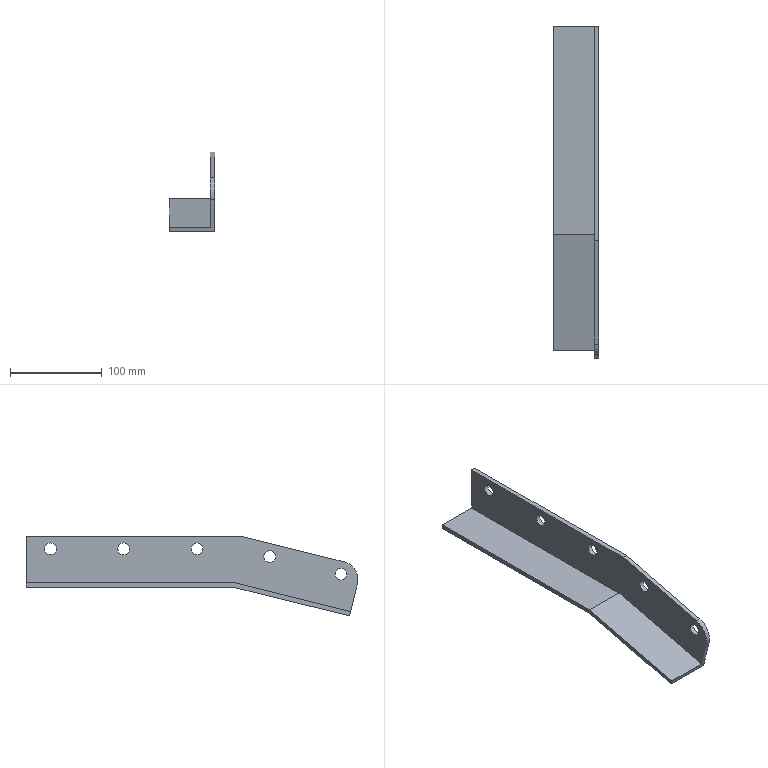Part | NX | features solid 2 | 1 solid | 17 faces | box 50 x 362.429 x 87.264 mm | volume 178588 mm3 | plane 11 | cylinder 6 | commonest cylinder face diameters 13 x5 40 x1
STEP:
#1=CARTESIAN_POINT('',(-584.258,-720.,106.));
#2=VERTEX_POINT('',#1);
#3=CARTESIAN_POINT('',(-584.258,-720.,55.));
#4=VERTEX_POINT('',#3);
#5=CARTESIAN_POINT('',(-584.258,-720.,85.));
#6=DIRECTION('',(0.,0.,-1.));
#7=VECTOR('',#6,1000.);
#8=LINE('',#5,#7);
#9=EDGE_CURVE('',#2,#4,#8,.T.);
#10=ORIENTED_EDGE('',*,*,#9,.F.);
#11=CARTESIAN_POINT('',(-579.258,-720.,106.));
#12=VERTEX_POINT('',#11);
#13=CARTESIAN_POINT('',(-584.258,-720.,106.));
#14=DIRECTION('',(-1.,0.,0.));
#15=VECTOR('',#14,1000.);
#16=LINE('',#13,#15);
#17=EDGE_CURVE('',#12,#2,#16,.T.);
#18=ORIENTED_EDGE('',*,*,#17,.F.);
#19=CARTESIAN_POINT('',(-579.258,-720.,50.));
#20=VERTEX_POINT('',#19);
#21=CARTESIAN_POINT('',(-579.258,-720.,85.));
#22=DIRECTION('',(0.,0.,1.));
#23=VECTOR('',#22,1000.);
#24=LINE('',#21,#23);
#25=EDGE_CURVE('',#20,#12,#24,.T.);
#26=ORIENTED_EDGE('',*,*,#25,.F.);
#27=CARTESIAN_POINT('',(-629.258,-720.,50.));
#28=VERTEX_POINT('',#27);
#29=CARTESIAN_POINT('',(-579.258,-720.,50.));
#30=DIRECTION('',(1.,0.,0.));
#31=VECTOR('',#30,1000.);
#32=LINE('',#29,#31);
#33=EDGE_CURVE('',#28,#20,#32,.T.);
#34=ORIENTED_EDGE('',*,*,#33,.F.);
#35=CARTESIAN_POINT('',(-629.258,-720.,55.));
#36=VERTEX_POINT('',#35);
#37=CARTESIAN_POINT('',(-629.258,-720.,85.));
#38=DIRECTION('',(0.,0.,-1.));
#39=VECTOR('',#38,1000.);
#40=LINE('',#37,#39);
#41=EDGE_CURVE('',#36,#28,#40,.T.);
#42=ORIENTED_EDGE('',*,*,#41,.F.);
#43=CARTESIAN_POINT('',(-624.258,-720.,55.));
#44=DIRECTION('',(-1.,0.,0.));
#45=VECTOR('',#44,1000.);
#46=LINE('',#43,#45);
#47=EDGE_CURVE('',#4,#36,#46,.T.);
#48=ORIENTED_EDGE('',*,*,#47,.F.);
#49=EDGE_LOOP('',(#10,#18,#26,#34,#42,#48));
#50=FACE_BOUND('',#49,.T.);
#51=CARTESIAN_POINT('',(-1045.,-720.,130.));
#52=DIRECTION('',(0.,1.,0.));
#53=DIRECTION('',(0.,0.,1.));
#54=AXIS2_PLACEMENT_3D('',#51,#52,#53);
#55=PLANE('',#54);
#56=ADVANCED_FACE('',(#50),#55,.T.);
#57=CARTESIAN_POINT('',(-584.258,-1063.872,70.813));
#58=VERTEX_POINT('',#57);
#59=CARTESIAN_POINT('',(-584.258,-1063.872,64.313));
#60=DIRECTION('',(1.,0.,0.));
#61=DIRECTION('',(0.,0.,1.));
#62=AXIS2_PLACEMENT_3D('',#59,#60,#61);
#63=CIRCLE('',#62,6.5);
#64=EDGE_CURVE('',#58,#58,#63,.T.);
#65=ORIENTED_EDGE('',*,*,#64,.T.);
#66=EDGE_LOOP('',(#65));
#67=FACE_BOUND('',#66,.T.);
#68=CARTESIAN_POINT('',(-584.258,-986.22,90.053));
#69=VERTEX_POINT('',#68);
#70=CARTESIAN_POINT('',(-584.258,-986.22,83.553));
#71=DIRECTION('',(1.,0.,0.));
#72=DIRECTION('',(0.,0.,1.));
#73=AXIS2_PLACEMENT_3D('',#70,#71,#72);
#74=CIRCLE('',#73,6.5);
#75=EDGE_CURVE('',#69,#69,#74,.T.);
#76=ORIENTED_EDGE('',*,*,#75,.T.);
#77=EDGE_LOOP('',(#76));
#78=FACE_BOUND('',#77,.T.);
#79=CARTESIAN_POINT('',(-584.258,-906.667,98.5));
#80=VERTEX_POINT('',#79);
#81=CARTESIAN_POINT('',(-584.258,-906.667,92.));
#82=DIRECTION('',(1.,0.,0.));
#83=DIRECTION('',(0.,0.,1.));
#84=AXIS2_PLACEMENT_3D('',#81,#82,#83);
#85=CIRCLE('',#84,6.5);
#86=EDGE_CURVE('',#80,#80,#85,.T.);
#87=ORIENTED_EDGE('',*,*,#86,.T.);
#88=EDGE_LOOP('',(#87));
#89=FACE_BOUND('',#88,.T.);
#90=CARTESIAN_POINT('',(-584.258,-826.667,98.5));
#91=VERTEX_POINT('',#90);
#92=CARTESIAN_POINT('',(-584.258,-826.667,92.));
#93=DIRECTION('',(1.,0.,0.));
#94=DIRECTION('',(0.,0.,1.));
#95=AXIS2_PLACEMENT_3D('',#92,#93,#94);
#96=CIRCLE('',#95,6.5);
#97=EDGE_CURVE('',#91,#91,#96,.T.);
#98=ORIENTED_EDGE('',*,*,#97,.T.);
#99=EDGE_LOOP('',(#98));
#100=FACE_BOUND('',#99,.T.);
#101=CARTESIAN_POINT('',(-584.258,-746.667,98.5));
#102=VERTEX_POINT('',#101);
#103=CARTESIAN_POINT('',(-584.258,-746.667,92.));
#104=DIRECTION('',(1.,0.,0.));
#105=DIRECTION('',(0.,0.,1.));
#106=AXIS2_PLACEMENT_3D('',#103,#104,#105);
#107=CIRCLE('',#106,6.5);
#108=EDGE_CURVE('',#102,#102,#107,.T.);
#109=ORIENTED_EDGE('',*,*,#108,.T.);
#110=EDGE_LOOP('',(#109));
#111=FACE_BOUND('',#110,.T.);
#112=CARTESIAN_POINT('',(-584.258,-953.834,106.));
#113=VERTEX_POINT('',#112);
#114=CARTESIAN_POINT('',(-584.258,-904.636,106.));
#115=DIRECTION('',(0.,-1.,0.));
#116=VECTOR('',#115,1000.);
#117=LINE('',#114,#116);
#118=EDGE_CURVE('',#2,#113,#117,.T.);
#119=ORIENTED_EDGE('',*,*,#118,.F.);
#120=ORIENTED_EDGE('',*,*,#9,.T.);
#121=CARTESIAN_POINT('',(-584.258,-947.61,55.));
#122=VERTEX_POINT('',#121);
#123=CARTESIAN_POINT('',(-584.258,-902.805,55.));
#124=DIRECTION('',(0.,-1.,0.));
#125=VECTOR('',#124,1000.);
#126=LINE('',#123,#125);
#127=EDGE_CURVE('',#4,#122,#126,.T.);
#128=ORIENTED_EDGE('',*,*,#127,.T.);
#129=CARTESIAN_POINT('',(-584.258,-1074.387,23.589));
#130=VERTEX_POINT('',#129);
#131=CARTESIAN_POINT('',(-584.258,-997.906,42.538));
#132=DIRECTION('',(0.,-0.9707,-0.2405));
#133=VECTOR('',#132,1000.);
#134=LINE('',#131,#133);
#135=EDGE_CURVE('',#122,#130,#134,.T.);
#136=ORIENTED_EDGE('',*,*,#135,.T.);
#137=CARTESIAN_POINT('',(-584.258,-1081.842,53.679));
#138=VERTEX_POINT('',#137);
#139=CARTESIAN_POINT('',(-584.258,-1073.185,18.736));
#140=DIRECTION('',(0.,0.2405,-0.9707));
#141=VECTOR('',#140,1000.);
#142=LINE('',#139,#141);
#143=EDGE_CURVE('',#138,#130,#142,.T.);
#144=ORIENTED_EDGE('',*,*,#143,.F.);
#145=CARTESIAN_POINT('',(-584.258,-1067.239,77.902));
#146=VERTEX_POINT('',#145);
#147=CARTESIAN_POINT('',(-584.258,-1062.429,58.489));
#148=DIRECTION('',(-1.,0.,0.));
#149=DIRECTION('',(0.,0.,-1.));
#150=AXIS2_PLACEMENT_3D('',#147,#148,#149);
#151=CIRCLE('',#150,20.);
#152=EDGE_CURVE('',#138,#146,#151,.T.);
#153=ORIENTED_EDGE('',*,*,#152,.T.);
#154=CARTESIAN_POINT('',(-584.258,-1008.395,92.482));
#155=DIRECTION('',(0.,-0.9707,-0.2405));
#156=VECTOR('',#155,1000.);
#157=LINE('',#154,#156);
#158=EDGE_CURVE('',#113,#146,#157,.T.);
#159=ORIENTED_EDGE('',*,*,#158,.F.);
#160=EDGE_LOOP('',(#119,#120,#128,#136,#144,#153,#159));
#161=FACE_BOUND('',#160,.T.);
#162=CARTESIAN_POINT('',(-584.258,-904.636,85.));
#163=DIRECTION('',(-1.,0.,0.));
#164=DIRECTION('',(0.,0.,-1.));
#165=AXIS2_PLACEMENT_3D('',#162,#163,#164);
#166=PLANE('',#165);
#167=ADVANCED_FACE('',(#67,#78,#89,#100,#111,#161),#166,.T.);
#168=CARTESIAN_POINT('',(-579.258,-1063.872,70.813));
#169=VERTEX_POINT('',#168);
#170=CARTESIAN_POINT('',(-579.258,-1063.872,64.313));
#171=DIRECTION('',(1.,0.,0.));
#172=DIRECTION('',(0.,0.,1.));
#173=AXIS2_PLACEMENT_3D('',#170,#171,#172);
#174=CIRCLE('',#173,6.5);
#175=EDGE_CURVE('',#169,#169,#174,.T.);
#176=ORIENTED_EDGE('',*,*,#175,.F.);
#177=EDGE_LOOP('',(#176));
#178=FACE_BOUND('',#177,.T.);
#179=CARTESIAN_POINT('',(-579.258,-986.22,90.053));
#180=VERTEX_POINT('',#179);
#181=CARTESIAN_POINT('',(-579.258,-986.22,83.553));
#182=DIRECTION('',(1.,0.,0.));
#183=DIRECTION('',(0.,0.,1.));
#184=AXIS2_PLACEMENT_3D('',#181,#182,#183);
#185=CIRCLE('',#184,6.5);
#186=EDGE_CURVE('',#180,#180,#185,.T.);
#187=ORIENTED_EDGE('',*,*,#186,.F.);
#188=EDGE_LOOP('',(#187));
#189=FACE_BOUND('',#188,.T.);
#190=CARTESIAN_POINT('',(-579.258,-906.667,98.5));
#191=VERTEX_POINT('',#190);
#192=CARTESIAN_POINT('',(-579.258,-906.667,92.));
#193=DIRECTION('',(1.,0.,0.));
#194=DIRECTION('',(0.,0.,1.));
#195=AXIS2_PLACEMENT_3D('',#192,#193,#194);
#196=CIRCLE('',#195,6.5);
#197=EDGE_CURVE('',#191,#191,#196,.T.);
#198=ORIENTED_EDGE('',*,*,#197,.F.);
#199=EDGE_LOOP('',(#198));
#200=FACE_BOUND('',#199,.T.);
#201=CARTESIAN_POINT('',(-579.258,-826.667,98.5));
#202=VERTEX_POINT('',#201);
#203=CARTESIAN_POINT('',(-579.258,-826.667,92.));
#204=DIRECTION('',(1.,0.,0.));
#205=DIRECTION('',(0.,0.,1.));
#206=AXIS2_PLACEMENT_3D('',#203,#204,#205);
#207=CIRCLE('',#206,6.5);
#208=EDGE_CURVE('',#202,#202,#207,.T.);
#209=ORIENTED_EDGE('',*,*,#208,.F.);
#210=EDGE_LOOP('',(#209));
#211=FACE_BOUND('',#210,.T.);
#212=CARTESIAN_POINT('',(-579.258,-746.667,98.5));
#213=VERTEX_POINT('',#212);
#214=CARTESIAN_POINT('',(-579.258,-746.667,92.));
#215=DIRECTION('',(1.,0.,0.));
#216=DIRECTION('',(0.,0.,1.));
#217=AXIS2_PLACEMENT_3D('',#214,#215,#216);
#218=CIRCLE('',#217,6.5);
#219=EDGE_CURVE('',#213,#213,#218,.T.);
#220=ORIENTED_EDGE('',*,*,#219,.F.);
#221=EDGE_LOOP('',(#220));
#222=FACE_BOUND('',#221,.T.);
#223=CARTESIAN_POINT('',(-579.258,-947.,50.));
#224=VERTEX_POINT('',#223);
#225=CARTESIAN_POINT('',(-579.258,-904.636,50.));
#226=DIRECTION('',(0.,1.,0.));
#227=VECTOR('',#226,1000.);
#228=LINE('',#225,#227);
#229=EDGE_CURVE('',#224,#20,#228,.T.);
#230=ORIENTED_EDGE('',*,*,#229,.T.);
#231=ORIENTED_EDGE('',*,*,#25,.T.);
#232=CARTESIAN_POINT('',(-579.258,-953.834,106.));
#233=VERTEX_POINT('',#232);
#234=CARTESIAN_POINT('',(-579.258,-904.636,106.));
#235=DIRECTION('',(0.,-1.,0.));
#236=VECTOR('',#235,1000.);
#237=LINE('',#234,#236);
#238=EDGE_CURVE('',#12,#233,#237,.T.);
#239=ORIENTED_EDGE('',*,*,#238,.T.);
#240=CARTESIAN_POINT('',(-579.258,-1067.239,77.902));
#241=VERTEX_POINT('',#240);
#242=CARTESIAN_POINT('',(-579.258,-912.383,116.27));
#243=DIRECTION('',(0.,-0.9707,-0.2405));
#244=VECTOR('',#243,1000.);
#245=LINE('',#242,#244);
#246=EDGE_CURVE('',#233,#241,#245,.T.);
#247=ORIENTED_EDGE('',*,*,#246,.T.);
#248=CARTESIAN_POINT('',(-579.258,-1081.842,53.679));
#249=VERTEX_POINT('',#248);
#250=CARTESIAN_POINT('',(-579.258,-1062.429,58.489));
#251=DIRECTION('',(1.,0.,0.));
#252=DIRECTION('',(0.,0.,1.));
#253=AXIS2_PLACEMENT_3D('',#250,#251,#252);
#254=CIRCLE('',#253,20.);
#255=EDGE_CURVE('',#241,#249,#254,.T.);
#256=ORIENTED_EDGE('',*,*,#255,.T.);
#257=CARTESIAN_POINT('',(-579.258,-1073.185,18.736));
#258=VERTEX_POINT('',#257);
#259=CARTESIAN_POINT('',(-579.258,-1073.185,18.736));
#260=DIRECTION('',(0.,-0.2405,0.9707));
#261=VECTOR('',#260,1000.);
#262=LINE('',#259,#261);
#263=EDGE_CURVE('',#258,#249,#262,.T.);
#264=ORIENTED_EDGE('',*,*,#263,.F.);
#265=CARTESIAN_POINT('',(-579.258,-997.,37.612));
#266=DIRECTION('',(0.,-0.9707,-0.2405));
#267=VECTOR('',#266,1000.);
#268=LINE('',#265,#267);
#269=EDGE_CURVE('',#224,#258,#268,.T.);
#270=ORIENTED_EDGE('',*,*,#269,.F.);
#271=EDGE_LOOP('',(#230,#231,#239,#247,#256,#264,#270));
#272=FACE_BOUND('',#271,.T.);
#273=CARTESIAN_POINT('',(-579.258,-904.636,85.));
#274=DIRECTION('',(1.,0.,0.));
#275=DIRECTION('',(0.,0.,1.));
#276=AXIS2_PLACEMENT_3D('',#273,#274,#275);
#277=PLANE('',#276);
#278=ADVANCED_FACE('',(#178,#189,#200,#211,#222,#272),#277,.T.);
#279=CARTESIAN_POINT('',(-629.258,-947.61,55.));
#280=VERTEX_POINT('',#279);
#281=CARTESIAN_POINT('',(-629.258,-904.636,55.));
#282=DIRECTION('',(0.,-1.,0.));
#283=VECTOR('',#282,1000.);
#284=LINE('',#281,#283);
#285=EDGE_CURVE('',#36,#280,#284,.T.);
#286=ORIENTED_EDGE('',*,*,#285,.F.);
#287=ORIENTED_EDGE('',*,*,#41,.T.);
#288=CARTESIAN_POINT('',(-629.258,-947.,50.));
#289=VERTEX_POINT('',#288);
#290=CARTESIAN_POINT('',(-629.258,-902.5,50.));
#291=DIRECTION('',(0.,-1.,0.));
#292=VECTOR('',#291,1000.);
#293=LINE('',#290,#292);
#294=EDGE_CURVE('',#28,#289,#293,.T.);
#295=ORIENTED_EDGE('',*,*,#294,.T.);
#296=CARTESIAN_POINT('',(-629.258,-1073.185,18.736));
#297=VERTEX_POINT('',#296);
#298=CARTESIAN_POINT('',(-629.258,-997.,37.612));
#299=DIRECTION('',(0.,-0.9707,-0.2405));
#300=VECTOR('',#299,1000.);
#301=LINE('',#298,#300);
#302=EDGE_CURVE('',#289,#297,#301,.T.);
#303=ORIENTED_EDGE('',*,*,#302,.T.);
#304=CARTESIAN_POINT('',(-629.258,-1074.387,23.589));
#305=VERTEX_POINT('',#304);
#306=CARTESIAN_POINT('',(-629.258,-1073.185,18.736));
#307=DIRECTION('',(0.,0.2405,-0.9707));
#308=VECTOR('',#307,1000.);
#309=LINE('',#306,#308);
#310=EDGE_CURVE('',#305,#297,#309,.T.);
#311=ORIENTED_EDGE('',*,*,#310,.F.);
#312=CARTESIAN_POINT('',(-629.258,-900.118,66.767));
#313=DIRECTION('',(0.,-0.9707,-0.2405));
#314=VECTOR('',#313,1000.);
#315=LINE('',#312,#314);
#316=EDGE_CURVE('',#280,#305,#315,.T.);
#317=ORIENTED_EDGE('',*,*,#316,.F.);
#318=EDGE_LOOP('',(#286,#287,#295,#303,#311,#317));
#319=FACE_BOUND('',#318,.T.);
#320=CARTESIAN_POINT('',(-629.258,-904.636,85.));
#321=DIRECTION('',(-1.,0.,0.));
#322=DIRECTION('',(0.,0.,-1.));
#323=AXIS2_PLACEMENT_3D('',#320,#321,#322);
#324=PLANE('',#323);
#325=ADVANCED_FACE('',(#319),#324,.T.);
#326=ORIENTED_EDGE('',*,*,#127,.F.);
#327=ORIENTED_EDGE('',*,*,#47,.T.);
#328=ORIENTED_EDGE('',*,*,#285,.T.);
#329=CARTESIAN_POINT('',(-604.258,-947.61,55.));
#330=DIRECTION('',(-1.,0.,0.));
#331=VECTOR('',#330,1000.);
#332=LINE('',#329,#331);
#333=EDGE_CURVE('',#122,#280,#332,.T.);
#334=ORIENTED_EDGE('',*,*,#333,.F.);
#335=EDGE_LOOP('',(#326,#327,#328,#334));
#336=FACE_BOUND('',#335,.T.);
#337=CARTESIAN_POINT('',(-624.258,-902.805,55.));
#338=DIRECTION('',(0.,0.,1.));
#339=DIRECTION('',(0.,-1.,0.));
#340=AXIS2_PLACEMENT_3D('',#337,#338,#339);
#341=PLANE('',#340);
#342=ADVANCED_FACE('',(#336),#341,.T.);
#343=ORIENTED_EDGE('',*,*,#238,.F.);
#344=ORIENTED_EDGE('',*,*,#17,.T.);
#345=ORIENTED_EDGE('',*,*,#118,.T.);
#346=CARTESIAN_POINT('',(-584.258,-953.834,106.));
#347=DIRECTION('',(-1.,0.,0.));
#348=VECTOR('',#347,1000.);
#349=LINE('',#346,#348);
#350=EDGE_CURVE('',#233,#113,#349,.T.);
#351=ORIENTED_EDGE('',*,*,#350,.F.);
#352=EDGE_LOOP('',(#343,#344,#345,#351));
#353=FACE_BOUND('',#352,.T.);
#354=CARTESIAN_POINT('',(-584.258,-904.636,106.));
#355=DIRECTION('',(0.,0.,1.));
#356=DIRECTION('',(0.,-1.,0.));
#357=AXIS2_PLACEMENT_3D('',#354,#355,#356);
#358=PLANE('',#357);
#359=ADVANCED_FACE('',(#353),#358,.T.);
#360=ORIENTED_EDGE('',*,*,#294,.F.);
#361=ORIENTED_EDGE('',*,*,#33,.T.);
#362=ORIENTED_EDGE('',*,*,#229,.F.);
#363=CARTESIAN_POINT('',(-604.258,-947.,50.));
#364=DIRECTION('',(1.,0.,0.));
#365=VECTOR('',#364,1000.);
#366=LINE('',#363,#365);
#367=EDGE_CURVE('',#289,#224,#366,.T.);
#368=ORIENTED_EDGE('',*,*,#367,.F.);
#369=EDGE_LOOP('',(#360,#361,#362,#368));
#370=FACE_BOUND('',#369,.T.);
#371=CARTESIAN_POINT('',(-579.258,-902.5,50.));
#372=DIRECTION('',(0.,0.,-1.));
#373=DIRECTION('',(0.,1.,0.));
#374=AXIS2_PLACEMENT_3D('',#371,#372,#373);
#375=PLANE('',#374);
#376=ADVANCED_FACE('',(#370),#375,.T.);
#377=ORIENTED_EDGE('',*,*,#263,.T.);
#378=CARTESIAN_POINT('',(-604.258,-1081.842,53.679));
#379=DIRECTION('',(-1.,0.,0.));
#380=VECTOR('',#379,1000.);
#381=LINE('',#378,#380);
#382=EDGE_CURVE('',#249,#138,#381,.T.);
#383=ORIENTED_EDGE('',*,*,#382,.T.);
#384=ORIENTED_EDGE('',*,*,#143,.T.);
#385=CARTESIAN_POINT('',(-604.258,-1074.387,23.589));
#386=DIRECTION('',(-1.,0.,0.));
#387=VECTOR('',#386,1000.);
#388=LINE('',#385,#387);
#389=EDGE_CURVE('',#130,#305,#388,.T.);
#390=ORIENTED_EDGE('',*,*,#389,.T.);
#391=ORIENTED_EDGE('',*,*,#310,.T.);
#392=CARTESIAN_POINT('',(-604.258,-1073.185,18.736));
#393=DIRECTION('',(1.,0.,0.));
#394=VECTOR('',#393,1000.);
#395=LINE('',#392,#394);
#396=EDGE_CURVE('',#297,#258,#395,.T.);
#397=ORIENTED_EDGE('',*,*,#396,.T.);
#398=EDGE_LOOP('',(#377,#383,#384,#390,#391,#397));
#399=FACE_BOUND('',#398,.T.);
#400=CARTESIAN_POINT('',(-604.258,-1073.185,18.736));
#401=DIRECTION('',(0.,-0.9707,-0.2405));
#402=DIRECTION('',(0.,0.2405,-0.9707));
#403=AXIS2_PLACEMENT_3D('',#400,#401,#402);
#404=PLANE('',#403);
#405=ADVANCED_FACE('',(#399),#404,.T.);
#406=ORIENTED_EDGE('',*,*,#316,.T.);
#407=ORIENTED_EDGE('',*,*,#389,.F.);
#408=ORIENTED_EDGE('',*,*,#135,.F.);
#409=ORIENTED_EDGE('',*,*,#333,.T.);
#410=EDGE_LOOP('',(#406,#407,#408,#409));
#411=FACE_BOUND('',#410,.T.);
#412=CARTESIAN_POINT('',(-624.258,-997.906,42.538));
#413=DIRECTION('',(0.,-0.2405,0.9707));
#414=DIRECTION('',(0.,-0.9707,-0.2405));
#415=AXIS2_PLACEMENT_3D('',#412,#413,#414);
#416=PLANE('',#415);
#417=ADVANCED_FACE('',(#411),#416,.T.);
#418=ORIENTED_EDGE('',*,*,#158,.T.);
#419=CARTESIAN_POINT('',(-584.258,-1067.239,77.902));
#420=DIRECTION('',(-1.,0.,0.));
#421=VECTOR('',#420,1000.);
#422=LINE('',#419,#421);
#423=EDGE_CURVE('',#146,#241,#422,.F.);
#424=ORIENTED_EDGE('',*,*,#423,.T.);
#425=ORIENTED_EDGE('',*,*,#246,.F.);
#426=ORIENTED_EDGE('',*,*,#350,.T.);
#427=EDGE_LOOP('',(#418,#424,#425,#426));
#428=FACE_BOUND('',#427,.T.);
#429=CARTESIAN_POINT('',(-584.258,-1008.395,92.482));
#430=DIRECTION('',(0.,-0.2405,0.9707));
#431=DIRECTION('',(0.,-0.9707,-0.2405));
#432=AXIS2_PLACEMENT_3D('',#429,#430,#431);
#433=PLANE('',#432);
#434=ADVANCED_FACE('',(#428),#433,.T.);
#435=ORIENTED_EDGE('',*,*,#302,.F.);
#436=ORIENTED_EDGE('',*,*,#367,.T.);
#437=ORIENTED_EDGE('',*,*,#269,.T.);
#438=ORIENTED_EDGE('',*,*,#396,.F.);
#439=EDGE_LOOP('',(#435,#436,#437,#438));
#440=FACE_BOUND('',#439,.T.);
#441=CARTESIAN_POINT('',(-579.258,-997.,37.612));
#442=DIRECTION('',(0.,0.2405,-0.9707));
#443=DIRECTION('',(0.,0.9707,0.2405));
#444=AXIS2_PLACEMENT_3D('',#441,#442,#443);
#445=PLANE('',#444);
#446=ADVANCED_FACE('',(#440),#445,.T.);
#447=ORIENTED_EDGE('',*,*,#175,.T.);
#448=EDGE_LOOP('',(#447));
#449=FACE_BOUND('',#448,.T.);
#450=ORIENTED_EDGE('',*,*,#64,.F.);
#451=EDGE_LOOP('',(#450));
#452=FACE_BOUND('',#451,.T.);
#453=CARTESIAN_POINT('',(-584.258,-1063.872,64.313));
#454=DIRECTION('',(1.,0.,0.));
#455=DIRECTION('',(0.,0.,1.));
#456=AXIS2_PLACEMENT_3D('',#453,#454,#455);
#457=CYLINDRICAL_SURFACE('',#456,6.5);
#458=ADVANCED_FACE('',(#449,#452),#457,.F.);
#459=ORIENTED_EDGE('',*,*,#186,.T.);
#460=EDGE_LOOP('',(#459));
#461=FACE_BOUND('',#460,.T.);
#462=ORIENTED_EDGE('',*,*,#75,.F.);
#463=EDGE_LOOP('',(#462));
#464=FACE_BOUND('',#463,.T.);
#465=CARTESIAN_POINT('',(-584.258,-986.22,83.553));
#466=DIRECTION('',(1.,0.,0.));
#467=DIRECTION('',(0.,0.,1.));
#468=AXIS2_PLACEMENT_3D('',#465,#466,#467);
#469=CYLINDRICAL_SURFACE('',#468,6.5);
#470=ADVANCED_FACE('',(#461,#464),#469,.F.);
#471=ORIENTED_EDGE('',*,*,#197,.T.);
#472=EDGE_LOOP('',(#471));
#473=FACE_BOUND('',#472,.T.);
#474=ORIENTED_EDGE('',*,*,#86,.F.);
#475=EDGE_LOOP('',(#474));
#476=FACE_BOUND('',#475,.T.);
#477=CARTESIAN_POINT('',(-584.258,-906.667,92.));
#478=DIRECTION('',(1.,0.,0.));
#479=DIRECTION('',(0.,0.,1.));
#480=AXIS2_PLACEMENT_3D('',#477,#478,#479);
#481=CYLINDRICAL_SURFACE('',#480,6.5);
#482=ADVANCED_FACE('',(#473,#476),#481,.F.);
#483=ORIENTED_EDGE('',*,*,#208,.T.);
#484=EDGE_LOOP('',(#483));
#485=FACE_BOUND('',#484,.T.);
#486=ORIENTED_EDGE('',*,*,#97,.F.);
#487=EDGE_LOOP('',(#486));
#488=FACE_BOUND('',#487,.T.);
#489=CARTESIAN_POINT('',(-584.258,-826.667,92.));
#490=DIRECTION('',(1.,0.,0.));
#491=DIRECTION('',(0.,0.,1.));
#492=AXIS2_PLACEMENT_3D('',#489,#490,#491);
#493=CYLINDRICAL_SURFACE('',#492,6.5);
#494=ADVANCED_FACE('',(#485,#488),#493,.F.);
#495=ORIENTED_EDGE('',*,*,#219,.T.);
#496=EDGE_LOOP('',(#495));
#497=FACE_BOUND('',#496,.T.);
#498=ORIENTED_EDGE('',*,*,#108,.F.);
#499=EDGE_LOOP('',(#498));
#500=FACE_BOUND('',#499,.T.);
#501=CARTESIAN_POINT('',(-584.258,-746.667,92.));
#502=DIRECTION('',(1.,0.,0.));
#503=DIRECTION('',(0.,0.,1.));
#504=AXIS2_PLACEMENT_3D('',#501,#502,#503);
#505=CYLINDRICAL_SURFACE('',#504,6.5);
#506=ADVANCED_FACE('',(#497,#500),#505,.F.);
#507=ORIENTED_EDGE('',*,*,#255,.F.);
#508=ORIENTED_EDGE('',*,*,#423,.F.);
#509=ORIENTED_EDGE('',*,*,#152,.F.);
#510=ORIENTED_EDGE('',*,*,#382,.F.);
#511=EDGE_LOOP('',(#507,#508,#509,#510));
#512=FACE_BOUND('',#511,.T.);
#513=CARTESIAN_POINT('',(-604.258,-1062.429,58.489));
#514=DIRECTION('',(-1.,0.,0.));
#515=DIRECTION('',(0.,0.,-1.));
#516=AXIS2_PLACEMENT_3D('',#513,#514,#515);
#517=CYLINDRICAL_SURFACE('',#516,20.);
#518=ADVANCED_FACE('',(#512),#517,.T.);
#519=CLOSED_SHELL('',(#56,#167,#278,#325,#342,#359,#376,#405,#417,#434,#446,#458,#470,#482,#494,#506,#518));
#520=MANIFOLD_SOLID_BREP('',#519);
#521=(LENGTH_UNIT()NAMED_UNIT(*)SI_UNIT(.MILLI.,.METRE.));
#522=UNCERTAINTY_MEASURE_WITH_UNIT(LENGTH_MEASURE(0.00001),#521,'','');
#523=(NAMED_UNIT(*)PLANE_ANGLE_UNIT()SI_UNIT($,.RADIAN.));
#524=(NAMED_UNIT(*)SI_UNIT($,.STERADIAN.)SOLID_ANGLE_UNIT());
#525=(GEOMETRIC_REPRESENTATION_CONTEXT(3)GLOBAL_UNCERTAINTY_ASSIGNED_CONTEXT((#522))GLOBAL_UNIT_ASSIGNED_CONTEXT((#521,#523,#524))REPRESENTATION_CONTEXT('',''));
#526=ADVANCED_BREP_SHAPE_REPRESENTATION('',(#520),#525);